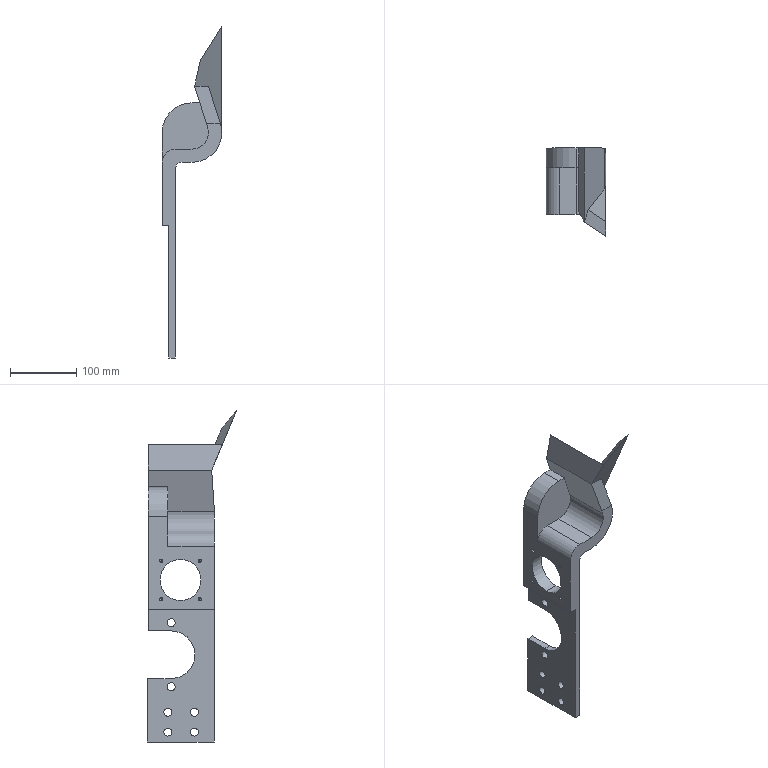Part | SolidWorks | features ICE 11, Extrusion 1, HoleWzd 1 | 1 solid | 65 faces | box 90 x 134.847 x 502.101 mm | volume 778867 mm3 | cylinder 32 | plane 25 | cone 8 | commonest cylinder face diameters 12 x12 5 x8 30 x2 62 x2 70 x2 90 x2